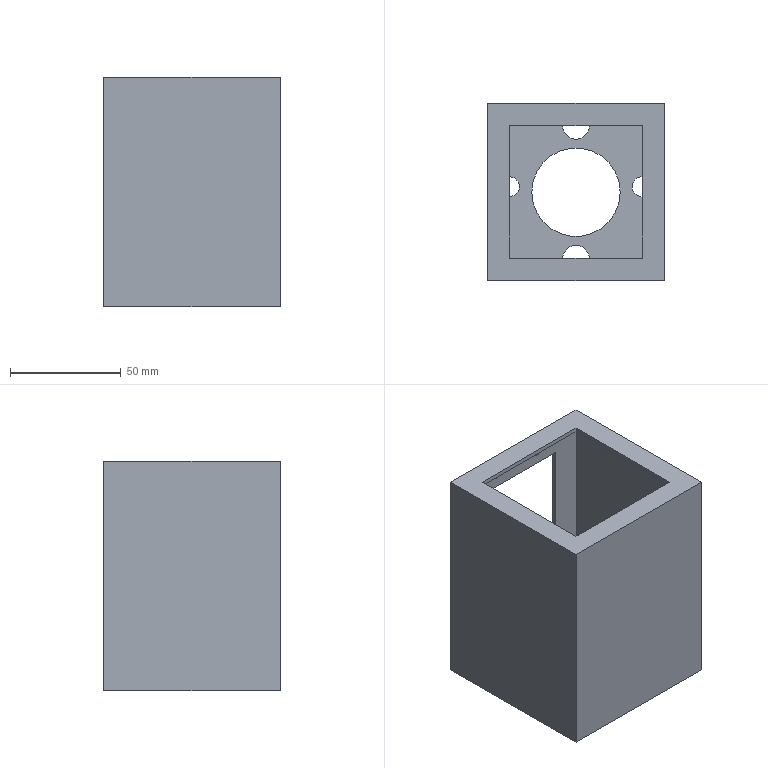Part | SolidWorks | features BaseBody 1 | 1 solid | 38 faces | box 80 x 80 x 104 mm | volume 72123 mm3 | plane 20 | cylinder 18 | commonest cylinder face diameters 3 x8 9 x4 12 x4 40 x2
STEP:
#1=CARTESIAN_POINT('',(6.,-30.,2.));
#2=VERTEX_POINT('',#1);
#3=CARTESIAN_POINT('',(-6.,-30.,2.));
#4=VERTEX_POINT('',#3);
#5=CARTESIAN_POINT('',(0.,-30.,2.));
#6=DIRECTION('',(0.,0.,-1.));
#7=DIRECTION('',(-1.,0.,0.));
#8=AXIS2_PLACEMENT_3D('',#5,#6,#7);
#9=CIRCLE('',#8,6.);
#10=EDGE_CURVE('',#2,#4,#9,.T.);
#11=ORIENTED_EDGE('',*,*,#10,.F.);
#12=CARTESIAN_POINT('',(6.,-30.,0.));
#13=VERTEX_POINT('',#12);
#14=CARTESIAN_POINT('',(6.,-30.,2.));
#15=DIRECTION('',(0.,0.,-1.));
#16=VECTOR('',#15,1000.);
#17=LINE('',#14,#16);
#18=EDGE_CURVE('',#2,#13,#17,.T.);
#19=ORIENTED_EDGE('',*,*,#18,.T.);
#20=CARTESIAN_POINT('',(-6.,-30.,0.));
#21=VERTEX_POINT('',#20);
#22=CARTESIAN_POINT('',(0.,-30.,0.));
#23=DIRECTION('',(0.,0.,1.));
#24=DIRECTION('',(-1.,0.,0.));
#25=AXIS2_PLACEMENT_3D('',#22,#23,#24);
#26=CIRCLE('',#25,6.);
#27=EDGE_CURVE('',#21,#13,#26,.T.);
#28=ORIENTED_EDGE('',*,*,#27,.F.);
#29=CARTESIAN_POINT('',(-6.,-30.,2.));
#30=DIRECTION('',(0.,0.,-1.));
#31=VECTOR('',#30,1000.);
#32=LINE('',#29,#31);
#33=EDGE_CURVE('',#4,#21,#32,.T.);
#34=ORIENTED_EDGE('',*,*,#33,.F.);
#35=EDGE_LOOP('',(#11,#19,#28,#34));
#36=FACE_OUTER_BOUND('',#35,.T.);
#37=CARTESIAN_POINT('',(0.,-30.,2.));
#38=DIRECTION('',(0.,0.,-1.));
#39=DIRECTION('',(-1.,0.,0.));
#40=AXIS2_PLACEMENT_3D('',#37,#38,#39);
#41=CYLINDRICAL_SURFACE('',#40,6.);
#42=ADVANCED_FACE('',(#36),#41,.F.);
#43=CARTESIAN_POINT('',(34.396,2.5,2.));
#44=VERTEX_POINT('',#43);
#45=CARTESIAN_POINT('',(25.396,2.5,2.));
#46=VERTEX_POINT('',#45);
#47=CARTESIAN_POINT('',(29.896,2.5,2.));
#48=DIRECTION('',(0.,0.,-1.));
#49=DIRECTION('',(-1.,0.,0.));
#50=AXIS2_PLACEMENT_3D('',#47,#48,#49);
#51=CIRCLE('',#50,4.5);
#52=EDGE_CURVE('',#44,#46,#51,.T.);
#53=ORIENTED_EDGE('',*,*,#52,.F.);
#54=CARTESIAN_POINT('',(34.396,2.5,0.));
#55=VERTEX_POINT('',#54);
#56=CARTESIAN_POINT('',(34.396,2.5,2.));
#57=DIRECTION('',(0.,0.,-1.));
#58=VECTOR('',#57,1000.);
#59=LINE('',#56,#58);
#60=EDGE_CURVE('',#44,#55,#59,.T.);
#61=ORIENTED_EDGE('',*,*,#60,.T.);
#62=CARTESIAN_POINT('',(25.396,2.5,0.));
#63=VERTEX_POINT('',#62);
#64=CARTESIAN_POINT('',(29.896,2.5,0.));
#65=DIRECTION('',(0.,0.,1.));
#66=DIRECTION('',(-1.,0.,0.));
#67=AXIS2_PLACEMENT_3D('',#64,#65,#66);
#68=CIRCLE('',#67,4.5);
#69=EDGE_CURVE('',#63,#55,#68,.T.);
#70=ORIENTED_EDGE('',*,*,#69,.F.);
#71=CARTESIAN_POINT('',(25.396,2.5,2.));
#72=DIRECTION('',(0.,0.,-1.));
#73=VECTOR('',#72,1000.);
#74=LINE('',#71,#73);
#75=EDGE_CURVE('',#46,#63,#74,.T.);
#76=ORIENTED_EDGE('',*,*,#75,.F.);
#77=EDGE_LOOP('',(#53,#61,#70,#76));
#78=FACE_OUTER_BOUND('',#77,.T.);
#79=CARTESIAN_POINT('',(29.896,2.5,2.));
#80=DIRECTION('',(0.,0.,-1.));
#81=DIRECTION('',(-1.,0.,0.));
#82=AXIS2_PLACEMENT_3D('',#79,#80,#81);
#83=CYLINDRICAL_SURFACE('',#82,4.5);
#84=ADVANCED_FACE('',(#78),#83,.F.);
#85=CARTESIAN_POINT('',(20.,0.,2.));
#86=VERTEX_POINT('',#85);
#87=CARTESIAN_POINT('',(-20.,0.,2.));
#88=VERTEX_POINT('',#87);
#89=CARTESIAN_POINT('',(0.,0.,2.));
#90=DIRECTION('',(0.,0.,-1.));
#91=DIRECTION('',(-1.,0.,0.));
#92=AXIS2_PLACEMENT_3D('',#89,#90,#91);
#93=CIRCLE('',#92,20.);
#94=EDGE_CURVE('',#86,#88,#93,.T.);
#95=ORIENTED_EDGE('',*,*,#94,.F.);
#96=CARTESIAN_POINT('',(20.,0.,0.));
#97=VERTEX_POINT('',#96);
#98=CARTESIAN_POINT('',(20.,0.,2.));
#99=DIRECTION('',(0.,0.,-1.));
#100=VECTOR('',#99,1000.);
#101=LINE('',#98,#100);
#102=EDGE_CURVE('',#86,#97,#101,.T.);
#103=ORIENTED_EDGE('',*,*,#102,.T.);
#104=CARTESIAN_POINT('',(-20.,0.,0.));
#105=VERTEX_POINT('',#104);
#106=CARTESIAN_POINT('',(0.,0.,0.));
#107=DIRECTION('',(0.,0.,1.));
#108=DIRECTION('',(-1.,0.,0.));
#109=AXIS2_PLACEMENT_3D('',#106,#107,#108);
#110=CIRCLE('',#109,20.);
#111=EDGE_CURVE('',#105,#97,#110,.T.);
#112=ORIENTED_EDGE('',*,*,#111,.F.);
#113=CARTESIAN_POINT('',(-20.,0.,2.));
#114=DIRECTION('',(0.,0.,-1.));
#115=VECTOR('',#114,1000.);
#116=LINE('',#113,#115);
#117=EDGE_CURVE('',#88,#105,#116,.T.);
#118=ORIENTED_EDGE('',*,*,#117,.F.);
#119=EDGE_LOOP('',(#95,#103,#112,#118));
#120=FACE_OUTER_BOUND('',#119,.T.);
#121=CARTESIAN_POINT('',(0.,0.,2.));
#122=DIRECTION('',(0.,0.,-1.));
#123=DIRECTION('',(-1.,0.,0.));
#124=AXIS2_PLACEMENT_3D('',#121,#122,#123);
#125=CYLINDRICAL_SURFACE('',#124,20.);
#126=ADVANCED_FACE('',(#120),#125,.F.);
#127=CARTESIAN_POINT('',(-25.604,2.5,2.));
#128=VERTEX_POINT('',#127);
#129=CARTESIAN_POINT('',(-34.604,2.5,2.));
#130=VERTEX_POINT('',#129);
#131=CARTESIAN_POINT('',(-30.104,2.5,2.));
#132=DIRECTION('',(0.,0.,-1.));
#133=DIRECTION('',(-1.,0.,0.));
#134=AXIS2_PLACEMENT_3D('',#131,#132,#133);
#135=CIRCLE('',#134,4.5);
#136=EDGE_CURVE('',#128,#130,#135,.T.);
#137=ORIENTED_EDGE('',*,*,#136,.F.);
#138=CARTESIAN_POINT('',(-25.604,2.5,0.));
#139=VERTEX_POINT('',#138);
#140=CARTESIAN_POINT('',(-25.604,2.5,2.));
#141=DIRECTION('',(0.,0.,-1.));
#142=VECTOR('',#141,1000.);
#143=LINE('',#140,#142);
#144=EDGE_CURVE('',#128,#139,#143,.T.);
#145=ORIENTED_EDGE('',*,*,#144,.T.);
#146=CARTESIAN_POINT('',(-34.604,2.5,0.));
#147=VERTEX_POINT('',#146);
#148=CARTESIAN_POINT('',(-30.104,2.5,0.));
#149=DIRECTION('',(0.,0.,1.));
#150=DIRECTION('',(-1.,0.,0.));
#151=AXIS2_PLACEMENT_3D('',#148,#149,#150);
#152=CIRCLE('',#151,4.5);
#153=EDGE_CURVE('',#147,#139,#152,.T.);
#154=ORIENTED_EDGE('',*,*,#153,.F.);
#155=CARTESIAN_POINT('',(-34.604,2.5,2.));
#156=DIRECTION('',(0.,0.,-1.));
#157=VECTOR('',#156,1000.);
#158=LINE('',#155,#157);
#159=EDGE_CURVE('',#130,#147,#158,.T.);
#160=ORIENTED_EDGE('',*,*,#159,.F.);
#161=EDGE_LOOP('',(#137,#145,#154,#160));
#162=FACE_OUTER_BOUND('',#161,.T.);
#163=CARTESIAN_POINT('',(-30.104,2.5,2.));
#164=DIRECTION('',(0.,0.,-1.));
#165=DIRECTION('',(-1.,0.,0.));
#166=AXIS2_PLACEMENT_3D('',#163,#164,#165);
#167=CYLINDRICAL_SURFACE('',#166,4.5);
#168=ADVANCED_FACE('',(#162),#167,.F.);
#169=CARTESIAN_POINT('',(6.,30.,2.));
#170=VERTEX_POINT('',#169);
#171=CARTESIAN_POINT('',(-6.,30.,2.));
#172=VERTEX_POINT('',#171);
#173=CARTESIAN_POINT('',(0.,30.,2.));
#174=DIRECTION('',(0.,0.,-1.));
#175=DIRECTION('',(-1.,0.,0.));
#176=AXIS2_PLACEMENT_3D('',#173,#174,#175);
#177=CIRCLE('',#176,6.);
#178=EDGE_CURVE('',#170,#172,#177,.T.);
#179=ORIENTED_EDGE('',*,*,#178,.F.);
#180=CARTESIAN_POINT('',(6.,30.,0.));
#181=VERTEX_POINT('',#180);
#182=CARTESIAN_POINT('',(6.,30.,2.));
#183=DIRECTION('',(0.,0.,-1.));
#184=VECTOR('',#183,1000.);
#185=LINE('',#182,#184);
#186=EDGE_CURVE('',#170,#181,#185,.T.);
#187=ORIENTED_EDGE('',*,*,#186,.T.);
#188=CARTESIAN_POINT('',(-6.,30.,0.));
#189=VERTEX_POINT('',#188);
#190=CARTESIAN_POINT('',(0.,30.,0.));
#191=DIRECTION('',(0.,0.,1.));
#192=DIRECTION('',(-1.,0.,0.));
#193=AXIS2_PLACEMENT_3D('',#190,#191,#192);
#194=CIRCLE('',#193,6.);
#195=EDGE_CURVE('',#189,#181,#194,.T.);
#196=ORIENTED_EDGE('',*,*,#195,.F.);
#197=CARTESIAN_POINT('',(-6.,30.,2.));
#198=DIRECTION('',(0.,0.,-1.));
#199=VECTOR('',#198,1000.);
#200=LINE('',#197,#199);
#201=EDGE_CURVE('',#172,#189,#200,.T.);
#202=ORIENTED_EDGE('',*,*,#201,.F.);
#203=EDGE_LOOP('',(#179,#187,#196,#202));
#204=FACE_OUTER_BOUND('',#203,.T.);
#205=CARTESIAN_POINT('',(0.,30.,2.));
#206=DIRECTION('',(0.,0.,-1.));
#207=DIRECTION('',(-1.,0.,0.));
#208=AXIS2_PLACEMENT_3D('',#205,#206,#207);
#209=CYLINDRICAL_SURFACE('',#208,6.);
#210=ADVANCED_FACE('',(#204),#209,.F.);
#211=CARTESIAN_POINT('',(-13.,38.,93.5));
#212=VERTEX_POINT('',#211);
#213=CARTESIAN_POINT('',(-13.,38.,96.5));
#214=VERTEX_POINT('',#213);
#215=CARTESIAN_POINT('',(-13.,38.,95.));
#216=DIRECTION('',(0.,1.,0.));
#217=DIRECTION('',(0.,0.,1.));
#218=AXIS2_PLACEMENT_3D('',#215,#216,#217);
#219=CIRCLE('',#218,1.5);
#220=EDGE_CURVE('',#212,#214,#219,.T.);
#221=ORIENTED_EDGE('',*,*,#220,.F.);
#222=CARTESIAN_POINT('',(-13.,40.,93.5));
#223=VERTEX_POINT('',#222);
#224=CARTESIAN_POINT('',(-13.,35.,93.5));
#225=DIRECTION('',(0.,1.,0.));
#226=VECTOR('',#225,1000.);
#227=LINE('',#224,#226);
#228=EDGE_CURVE('',#212,#223,#227,.T.);
#229=ORIENTED_EDGE('',*,*,#228,.T.);
#230=CARTESIAN_POINT('',(-13.,40.,96.5));
#231=VERTEX_POINT('',#230);
#232=CARTESIAN_POINT('',(-13.,40.,95.));
#233=DIRECTION('',(0.,1.,0.));
#234=DIRECTION('',(0.,0.,1.));
#235=AXIS2_PLACEMENT_3D('',#232,#233,#234);
#236=CIRCLE('',#235,1.5);
#237=EDGE_CURVE('',#223,#231,#236,.T.);
#238=ORIENTED_EDGE('',*,*,#237,.T.);
#239=CARTESIAN_POINT('',(-13.,35.,96.5));
#240=DIRECTION('',(0.,1.,0.));
#241=VECTOR('',#240,1000.);
#242=LINE('',#239,#241);
#243=EDGE_CURVE('',#214,#231,#242,.T.);
#244=ORIENTED_EDGE('',*,*,#243,.F.);
#245=EDGE_LOOP('',(#221,#229,#238,#244));
#246=FACE_OUTER_BOUND('',#245,.T.);
#247=CARTESIAN_POINT('',(-13.,35.,95.));
#248=DIRECTION('',(0.,1.,0.));
#249=DIRECTION('',(0.,0.,1.));
#250=AXIS2_PLACEMENT_3D('',#247,#248,#249);
#251=CYLINDRICAL_SURFACE('',#250,1.5);
#252=ADVANCED_FACE('',(#246),#251,.F.);
#253=CARTESIAN_POINT('',(13.,38.,93.5));
#254=VERTEX_POINT('',#253);
#255=CARTESIAN_POINT('',(13.,38.,96.5));
#256=VERTEX_POINT('',#255);
#257=CARTESIAN_POINT('',(13.,38.,95.));
#258=DIRECTION('',(0.,1.,0.));
#259=DIRECTION('',(0.,0.,1.));
#260=AXIS2_PLACEMENT_3D('',#257,#258,#259);
#261=CIRCLE('',#260,1.5);
#262=EDGE_CURVE('',#254,#256,#261,.T.);
#263=ORIENTED_EDGE('',*,*,#262,.F.);
#264=CARTESIAN_POINT('',(13.,40.,93.5));
#265=VERTEX_POINT('',#264);
#266=CARTESIAN_POINT('',(13.,35.,93.5));
#267=DIRECTION('',(0.,1.,0.));
#268=VECTOR('',#267,1000.);
#269=LINE('',#266,#268);
#270=EDGE_CURVE('',#254,#265,#269,.T.);
#271=ORIENTED_EDGE('',*,*,#270,.T.);
#272=CARTESIAN_POINT('',(13.,40.,96.5));
#273=VERTEX_POINT('',#272);
#274=CARTESIAN_POINT('',(13.,40.,95.));
#275=DIRECTION('',(0.,1.,0.));
#276=DIRECTION('',(0.,0.,1.));
#277=AXIS2_PLACEMENT_3D('',#274,#275,#276);
#278=CIRCLE('',#277,1.5);
#279=EDGE_CURVE('',#265,#273,#278,.T.);
#280=ORIENTED_EDGE('',*,*,#279,.T.);
#281=CARTESIAN_POINT('',(13.,35.,96.5));
#282=DIRECTION('',(0.,1.,0.));
#283=VECTOR('',#282,1000.);
#284=LINE('',#281,#283);
#285=EDGE_CURVE('',#256,#273,#284,.T.);
#286=ORIENTED_EDGE('',*,*,#285,.F.);
#287=EDGE_LOOP('',(#263,#271,#280,#286));
#288=FACE_OUTER_BOUND('',#287,.T.);
#289=CARTESIAN_POINT('',(13.,35.,95.));
#290=DIRECTION('',(0.,1.,0.));
#291=DIRECTION('',(0.,0.,1.));
#292=AXIS2_PLACEMENT_3D('',#289,#290,#291);
#293=CYLINDRICAL_SURFACE('',#292,1.5);
#294=ADVANCED_FACE('',(#288),#293,.F.);
#295=CARTESIAN_POINT('',(13.,38.,27.5));
#296=VERTEX_POINT('',#295);
#297=CARTESIAN_POINT('',(13.,38.,30.5));
#298=VERTEX_POINT('',#297);
#299=CARTESIAN_POINT('',(13.,38.,29.));
#300=DIRECTION('',(0.,1.,0.));
#301=DIRECTION('',(0.,0.,1.));
#302=AXIS2_PLACEMENT_3D('',#299,#300,#301);
#303=CIRCLE('',#302,1.5);
#304=EDGE_CURVE('',#296,#298,#303,.T.);
#305=ORIENTED_EDGE('',*,*,#304,.F.);
#306=CARTESIAN_POINT('',(13.,40.,27.5));
#307=VERTEX_POINT('',#306);
#308=CARTESIAN_POINT('',(13.,35.,27.5));
#309=DIRECTION('',(0.,1.,0.));
#310=VECTOR('',#309,1000.);
#311=LINE('',#308,#310);
#312=EDGE_CURVE('',#296,#307,#311,.T.);
#313=ORIENTED_EDGE('',*,*,#312,.T.);
#314=CARTESIAN_POINT('',(13.,40.,30.5));
#315=VERTEX_POINT('',#314);
#316=CARTESIAN_POINT('',(13.,40.,29.));
#317=DIRECTION('',(0.,1.,0.));
#318=DIRECTION('',(0.,0.,1.));
#319=AXIS2_PLACEMENT_3D('',#316,#317,#318);
#320=CIRCLE('',#319,1.5);
#321=EDGE_CURVE('',#307,#315,#320,.T.);
#322=ORIENTED_EDGE('',*,*,#321,.T.);
#323=CARTESIAN_POINT('',(13.,35.,30.5));
#324=DIRECTION('',(0.,1.,0.));
#325=VECTOR('',#324,1000.);
#326=LINE('',#323,#325);
#327=EDGE_CURVE('',#298,#315,#326,.T.);
#328=ORIENTED_EDGE('',*,*,#327,.F.);
#329=EDGE_LOOP('',(#305,#313,#322,#328));
#330=FACE_OUTER_BOUND('',#329,.T.);
#331=CARTESIAN_POINT('',(13.,35.,29.));
#332=DIRECTION('',(0.,1.,0.));
#333=DIRECTION('',(0.,0.,1.));
#334=AXIS2_PLACEMENT_3D('',#331,#332,#333);
#335=CYLINDRICAL_SURFACE('',#334,1.5);
#336=ADVANCED_FACE('',(#330),#335,.F.);
#337=CARTESIAN_POINT('',(-13.,38.,27.5));
#338=VERTEX_POINT('',#337);
#339=CARTESIAN_POINT('',(-13.,38.,30.5));
#340=VERTEX_POINT('',#339);
#341=CARTESIAN_POINT('',(-13.,38.,29.));
#342=DIRECTION('',(0.,1.,0.));
#343=DIRECTION('',(0.,0.,1.));
#344=AXIS2_PLACEMENT_3D('',#341,#342,#343);
#345=CIRCLE('',#344,1.5);
#346=EDGE_CURVE('',#338,#340,#345,.T.);
#347=ORIENTED_EDGE('',*,*,#346,.F.);
#348=CARTESIAN_POINT('',(-13.,40.,27.5));
#349=VERTEX_POINT('',#348);
#350=CARTESIAN_POINT('',(-13.,35.,27.5));
#351=DIRECTION('',(0.,1.,0.));
#352=VECTOR('',#351,1000.);
#353=LINE('',#350,#352);
#354=EDGE_CURVE('',#338,#349,#353,.T.);
#355=ORIENTED_EDGE('',*,*,#354,.T.);
#356=CARTESIAN_POINT('',(-13.,40.,30.5));
#357=VERTEX_POINT('',#356);
#358=CARTESIAN_POINT('',(-13.,40.,29.));
#359=DIRECTION('',(0.,1.,0.));
#360=DIRECTION('',(0.,0.,1.));
#361=AXIS2_PLACEMENT_3D('',#358,#359,#360);
#362=CIRCLE('',#361,1.5);
#363=EDGE_CURVE('',#349,#357,#362,.T.);
#364=ORIENTED_EDGE('',*,*,#363,.T.);
#365=CARTESIAN_POINT('',(-13.,35.,30.5));
#366=DIRECTION('',(0.,1.,0.));
#367=VECTOR('',#366,1000.);
#368=LINE('',#365,#367);
#369=EDGE_CURVE('',#340,#357,#368,.T.);
#370=ORIENTED_EDGE('',*,*,#369,.F.);
#371=EDGE_LOOP('',(#347,#355,#364,#370));
#372=FACE_OUTER_BOUND('',#371,.T.);
#373=CARTESIAN_POINT('',(-13.,35.,29.));
#374=DIRECTION('',(0.,1.,0.));
#375=DIRECTION('',(0.,0.,1.));
#376=AXIS2_PLACEMENT_3D('',#373,#374,#375);
#377=CYLINDRICAL_SURFACE('',#376,1.5);
#378=ADVANCED_FACE('',(#372),#377,.F.);
#379=CARTESIAN_POINT('',(-40.,-40.,104.));
#380=VERTEX_POINT('',#379);
#381=CARTESIAN_POINT('',(-40.,-40.,0.));
#382=VERTEX_POINT('',#381);
#383=CARTESIAN_POINT('',(-40.,-40.,2.));
#384=DIRECTION('',(0.,0.,-1.));
#385=VECTOR('',#384,1000.);
#386=LINE('',#383,#385);
#387=EDGE_CURVE('',#380,#382,#386,.T.);
#388=ORIENTED_EDGE('',*,*,#387,.F.);
#389=CARTESIAN_POINT('',(-40.,40.,104.));
#390=VERTEX_POINT('',#389);
#391=CARTESIAN_POINT('',(-40.,40.,104.));
#392=DIRECTION('',(0.,-1.,0.));
#393=VECTOR('',#392,1000.);
#394=LINE('',#391,#393);
#395=EDGE_CURVE('',#390,#380,#394,.T.);
#396=ORIENTED_EDGE('',*,*,#395,.F.);
#397=CARTESIAN_POINT('',(-40.,40.,0.));
#398=VERTEX_POINT('',#397);
#399=CARTESIAN_POINT('',(-40.,40.,2.));
#400=DIRECTION('',(0.,0.,1.));
#401=VECTOR('',#400,1000.);
#402=LINE('',#399,#401);
#403=EDGE_CURVE('',#398,#390,#402,.T.);
#404=ORIENTED_EDGE('',*,*,#403,.F.);
#405=CARTESIAN_POINT('',(-40.,40.,0.));
#406=DIRECTION('',(0.,1.,0.));
#407=VECTOR('',#406,1000.);
#408=LINE('',#405,#407);
#409=EDGE_CURVE('',#382,#398,#408,.T.);
#410=ORIENTED_EDGE('',*,*,#409,.F.);
#411=EDGE_LOOP('',(#388,#396,#404,#410));
#412=FACE_OUTER_BOUND('',#411,.T.);
#413=CARTESIAN_POINT('',(-40.,40.,2.));
#414=DIRECTION('',(1.,0.,0.));
#415=DIRECTION('',(0.,1.,0.));
#416=AXIS2_PLACEMENT_3D('',#413,#414,#415);
#417=PLANE('',#416);
#418=ADVANCED_FACE('',(#412),#417,.F.);
#419=ORIENTED_EDGE('',*,*,#27,.T.);
#420=CARTESIAN_POINT('',(0.,-30.,0.));
#421=DIRECTION('',(0.,0.,1.));
#422=DIRECTION('',(-1.,0.,0.));
#423=AXIS2_PLACEMENT_3D('',#420,#421,#422);
#424=CIRCLE('',#423,6.);
#425=EDGE_CURVE('',#13,#21,#424,.T.);
#426=ORIENTED_EDGE('',*,*,#425,.T.);
#427=EDGE_LOOP('',(#419,#426));
#428=FACE_BOUND('',#427,.T.);
#429=ORIENTED_EDGE('',*,*,#69,.T.);
#430=CARTESIAN_POINT('',(29.896,2.5,0.));
#431=DIRECTION('',(0.,0.,1.));
#432=DIRECTION('',(-1.,0.,0.));
#433=AXIS2_PLACEMENT_3D('',#430,#431,#432);
#434=CIRCLE('',#433,4.5);
#435=EDGE_CURVE('',#55,#63,#434,.T.);
#436=ORIENTED_EDGE('',*,*,#435,.T.);
#437=EDGE_LOOP('',(#429,#436));
#438=FACE_BOUND('',#437,.T.);
#439=ORIENTED_EDGE('',*,*,#111,.T.);
#440=CARTESIAN_POINT('',(0.,0.,0.));
#441=DIRECTION('',(0.,0.,1.));
#442=DIRECTION('',(-1.,0.,0.));
#443=AXIS2_PLACEMENT_3D('',#440,#441,#442);
#444=CIRCLE('',#443,20.);
#445=EDGE_CURVE('',#97,#105,#444,.T.);
#446=ORIENTED_EDGE('',*,*,#445,.T.);
#447=EDGE_LOOP('',(#439,#446));
#448=FACE_BOUND('',#447,.T.);
#449=ORIENTED_EDGE('',*,*,#153,.T.);
#450=CARTESIAN_POINT('',(-30.104,2.5,0.));
#451=DIRECTION('',(0.,0.,1.));
#452=DIRECTION('',(-1.,0.,0.));
#453=AXIS2_PLACEMENT_3D('',#450,#451,#452);
#454=CIRCLE('',#453,4.5);
#455=EDGE_CURVE('',#139,#147,#454,.T.);
#456=ORIENTED_EDGE('',*,*,#455,.T.);
#457=EDGE_LOOP('',(#449,#456));
#458=FACE_BOUND('',#457,.T.);
#459=ORIENTED_EDGE('',*,*,#195,.T.);
#460=CARTESIAN_POINT('',(0.,30.,0.));
#461=DIRECTION('',(0.,0.,1.));
#462=DIRECTION('',(-1.,0.,0.));
#463=AXIS2_PLACEMENT_3D('',#460,#461,#462);
#464=CIRCLE('',#463,6.);
#465=EDGE_CURVE('',#181,#189,#464,.T.);
#466=ORIENTED_EDGE('',*,*,#465,.T.);
#467=EDGE_LOOP('',(#459,#466));
#468=FACE_BOUND('',#467,.T.);
#469=CARTESIAN_POINT('',(40.,40.,0.));
#470=VERTEX_POINT('',#469);
#471=CARTESIAN_POINT('',(40.,-40.,0.));
#472=VERTEX_POINT('',#471);
#473=CARTESIAN_POINT('',(40.,0.,0.));
#474=DIRECTION('',(0.,-1.,0.));
#475=VECTOR('',#474,1000.);
#476=LINE('',#473,#475);
#477=EDGE_CURVE('',#470,#472,#476,.T.);
#478=ORIENTED_EDGE('',*,*,#477,.T.);
#479=CARTESIAN_POINT('',(0.,-40.,0.));
#480=DIRECTION('',(-1.,0.,0.));
#481=VECTOR('',#480,1000.);
#482=LINE('',#479,#481);
#483=EDGE_CURVE('',#472,#382,#482,.T.);
#484=ORIENTED_EDGE('',*,*,#483,.T.);
#485=ORIENTED_EDGE('',*,*,#409,.T.);
#486=CARTESIAN_POINT('',(0.,40.,0.));
#487=DIRECTION('',(1.,0.,0.));
#488=VECTOR('',#487,1000.);
#489=LINE('',#486,#488);
#490=EDGE_CURVE('',#398,#470,#489,.T.);
#491=ORIENTED_EDGE('',*,*,#490,.T.);
#492=EDGE_LOOP('',(#478,#484,#485,#491));
#493=FACE_OUTER_BOUND('',#492,.T.);
#494=CARTESIAN_POINT('',(0.,0.,0.));
#495=DIRECTION('',(0.,0.,-1.));
#496=DIRECTION('',(-1.,0.,0.));
#497=AXIS2_PLACEMENT_3D('',#494,#495,#496);
#498=PLANE('',#497);
#499=ADVANCED_FACE('',(#428,#438,#448,#458,#468,#493),#498,.T.);
#500=CARTESIAN_POINT('',(40.,-40.,104.));
#501=VERTEX_POINT('',#500);
#502=CARTESIAN_POINT('',(40.,-40.,2.));
#503=DIRECTION('',(0.,0.,-1.));
#504=VECTOR('',#503,1000.);
#505=LINE('',#502,#504);
#506=EDGE_CURVE('',#501,#472,#505,.T.);
#507=ORIENTED_EDGE('',*,*,#506,.F.);
#508=CARTESIAN_POINT('',(40.,-40.,104.));
#509=DIRECTION('',(1.,0.,0.));
#510=VECTOR('',#509,1000.);
#511=LINE('',#508,#510);
#512=EDGE_CURVE('',#380,#501,#511,.T.);
#513=ORIENTED_EDGE('',*,*,#512,.F.);
#514=ORIENTED_EDGE('',*,*,#387,.T.);
#515=ORIENTED_EDGE('',*,*,#483,.F.);
#516=EDGE_LOOP('',(#507,#513,#514,#515));
#517=FACE_OUTER_BOUND('',#516,.T.);
#518=CARTESIAN_POINT('',(40.,-40.,2.));
#519=DIRECTION('',(0.,1.,0.));
#520=DIRECTION('',(-1.,0.,0.));
#521=AXIS2_PLACEMENT_3D('',#518,#519,#520);
#522=PLANE('',#521);
#523=ADVANCED_FACE('',(#517),#522,.F.);
#524=CARTESIAN_POINT('',(-30.,30.,104.));
#525=VERTEX_POINT('',#524);
#526=CARTESIAN_POINT('',(30.,30.,104.));
#527=VERTEX_POINT('',#526);
#528=CARTESIAN_POINT('',(0.,30.,104.));
#529=DIRECTION('',(1.,0.,0.));
#530=VECTOR('',#529,1000.);
#531=LINE('',#528,#530);
#532=EDGE_CURVE('',#525,#527,#531,.T.);
#533=ORIENTED_EDGE('',*,*,#532,.T.);
#534=CARTESIAN_POINT('',(30.,-30.,104.));
#535=VERTEX_POINT('',#534);
#536=CARTESIAN_POINT('',(30.,0.,104.));
#537=DIRECTION('',(0.,-1.,0.));
#538=VECTOR('',#537,1000.);
#539=LINE('',#536,#538);
#540=EDGE_CURVE('',#527,#535,#539,.T.);
#541=ORIENTED_EDGE('',*,*,#540,.T.);
#542=CARTESIAN_POINT('',(-30.,-30.,104.));
#543=VERTEX_POINT('',#542);
#544=CARTESIAN_POINT('',(0.,-30.,104.));
#545=DIRECTION('',(-1.,0.,0.));
#546=VECTOR('',#545,1000.);
#547=LINE('',#544,#546);
#548=EDGE_CURVE('',#535,#543,#547,.T.);
#549=ORIENTED_EDGE('',*,*,#548,.T.);
#550=CARTESIAN_POINT('',(-30.,0.,104.));
#551=DIRECTION('',(0.,1.,0.));
#552=VECTOR('',#551,1000.);
#553=LINE('',#550,#552);
#554=EDGE_CURVE('',#543,#525,#553,.T.);
#555=ORIENTED_EDGE('',*,*,#554,.T.);
#556=EDGE_LOOP('',(#533,#541,#549,#555));
#557=FACE_BOUND('',#556,.T.);
#558=CARTESIAN_POINT('',(40.,40.,104.));
#559=VERTEX_POINT('',#558);
#560=CARTESIAN_POINT('',(40.,0.,104.));
#561=DIRECTION('',(0.,1.,0.));
#562=VECTOR('',#561,1000.);
#563=LINE('',#560,#562);
#564=EDGE_CURVE('',#501,#559,#563,.T.);
#565=ORIENTED_EDGE('',*,*,#564,.T.);
#566=CARTESIAN_POINT('',(0.,40.,104.));
#567=DIRECTION('',(-1.,0.,0.));
#568=VECTOR('',#567,1000.);
#569=LINE('',#566,#568);
#570=EDGE_CURVE('',#559,#390,#569,.T.);
#571=ORIENTED_EDGE('',*,*,#570,.T.);
#572=ORIENTED_EDGE('',*,*,#395,.T.);
#573=ORIENTED_EDGE('',*,*,#512,.T.);
#574=EDGE_LOOP('',(#565,#571,#572,#573));
#575=FACE_OUTER_BOUND('',#574,.T.);
#576=CARTESIAN_POINT('',(0.,0.,104.));
#577=DIRECTION('',(0.,0.,1.));
#578=DIRECTION('',(1.,0.,0.));
#579=AXIS2_PLACEMENT_3D('',#576,#577,#578);
#580=PLANE('',#579);
#581=ADVANCED_FACE('',(#557,#575),#580,.T.);
#582=CARTESIAN_POINT('',(-25.,40.,35.));
#583=VERTEX_POINT('',#582);
#584=CARTESIAN_POINT('',(-25.,40.,89.));
#585=VERTEX_POINT('',#584);
#586=CARTESIAN_POINT('',(-25.,40.,2.));
#587=DIRECTION('',(0.,0.,1.));
#588=VECTOR('',#587,1000.);
#589=LINE('',#586,#588);
#590=EDGE_CURVE('',#583,#585,#589,.T.);
#591=ORIENTED_EDGE('',*,*,#590,.F.);
#592=CARTESIAN_POINT('',(25.,40.,35.));
#593=VERTEX_POINT('',#592);
#594=CARTESIAN_POINT('',(40.,40.,35.));
#595=DIRECTION('',(-1.,0.,0.));
#596=VECTOR('',#595,1000.);
#597=LINE('',#594,#596);
#598=EDGE_CURVE('',#593,#583,#597,.T.);
#599=ORIENTED_EDGE('',*,*,#598,.F.);
#600=CARTESIAN_POINT('',(25.,40.,89.));
#601=VERTEX_POINT('',#600);
#602=CARTESIAN_POINT('',(25.,40.,2.));
#603=DIRECTION('',(0.,0.,-1.));
#604=VECTOR('',#603,1000.);
#605=LINE('',#602,#604);
#606=EDGE_CURVE('',#601,#593,#605,.T.);
#607=ORIENTED_EDGE('',*,*,#606,.F.);
#608=CARTESIAN_POINT('',(40.,40.,89.));
#609=DIRECTION('',(1.,0.,0.));
#610=VECTOR('',#609,1000.);
#611=LINE('',#608,#610);
#612=EDGE_CURVE('',#585,#601,#611,.T.);
#613=ORIENTED_EDGE('',*,*,#612,.F.);
#614=EDGE_LOOP('',(#591,#599,#607,#613));
#615=FACE_BOUND('',#614,.T.);
#616=CARTESIAN_POINT('',(-13.,40.,95.));
#617=DIRECTION('',(0.,1.,0.));
#618=DIRECTION('',(0.,0.,1.));
#619=AXIS2_PLACEMENT_3D('',#616,#617,#618);
#620=CIRCLE('',#619,1.5);
#621=EDGE_CURVE('',#231,#223,#620,.T.);
#622=ORIENTED_EDGE('',*,*,#621,.F.);
#623=ORIENTED_EDGE('',*,*,#237,.F.);
#624=EDGE_LOOP('',(#622,#623));
#625=FACE_BOUND('',#624,.T.);
#626=CARTESIAN_POINT('',(13.,40.,95.));
#627=DIRECTION('',(0.,1.,0.));
#628=DIRECTION('',(0.,0.,1.));
#629=AXIS2_PLACEMENT_3D('',#626,#627,#628);
#630=CIRCLE('',#629,1.5);
#631=EDGE_CURVE('',#273,#265,#630,.T.);
#632=ORIENTED_EDGE('',*,*,#631,.F.);
#633=ORIENTED_EDGE('',*,*,#279,.F.);
#634=EDGE_LOOP('',(#632,#633));
#635=FACE_BOUND('',#634,.T.);
#636=CARTESIAN_POINT('',(13.,40.,29.));
#637=DIRECTION('',(0.,1.,0.));
#638=DIRECTION('',(0.,0.,1.));
#639=AXIS2_PLACEMENT_3D('',#636,#637,#638);
#640=CIRCLE('',#639,1.5);
#641=EDGE_CURVE('',#315,#307,#640,.T.);
#642=ORIENTED_EDGE('',*,*,#641,.F.);
#643=ORIENTED_EDGE('',*,*,#321,.F.);
#644=EDGE_LOOP('',(#642,#643));
#645=FACE_BOUND('',#644,.T.);
#646=CARTESIAN_POINT('',(-13.,40.,29.));
#647=DIRECTION('',(0.,1.,0.));
#648=DIRECTION('',(0.,0.,1.));
#649=AXIS2_PLACEMENT_3D('',#646,#647,#648);
#650=CIRCLE('',#649,1.5);
#651=EDGE_CURVE('',#357,#349,#650,.T.);
#652=ORIENTED_EDGE('',*,*,#651,.F.);
#653=ORIENTED_EDGE('',*,*,#363,.F.);
#654=EDGE_LOOP('',(#652,#653));
#655=FACE_BOUND('',#654,.T.);
#656=ORIENTED_EDGE('',*,*,#403,.T.);
#657=ORIENTED_EDGE('',*,*,#570,.F.);
#658=CARTESIAN_POINT('',(40.,40.,2.));
#659=DIRECTION('',(0.,0.,1.));
#660=VECTOR('',#659,1000.);
#661=LINE('',#658,#660);
#662=EDGE_CURVE('',#470,#559,#661,.T.);
#663=ORIENTED_EDGE('',*,*,#662,.F.);
#664=ORIENTED_EDGE('',*,*,#490,.F.);
#665=EDGE_LOOP('',(#656,#657,#663,#664));
#666=FACE_OUTER_BOUND('',#665,.T.);
#667=CARTESIAN_POINT('',(40.,40.,2.));
#668=DIRECTION('',(0.,-1.,0.));
#669=DIRECTION('',(1.,0.,0.));
#670=AXIS2_PLACEMENT_3D('',#667,#668,#669);
#671=PLANE('',#670);
#672=ADVANCED_FACE('',(#615,#625,#635,#645,#655,#666),#671,.F.);
#673=ORIENTED_EDGE('',*,*,#18,.F.);
#674=CARTESIAN_POINT('',(0.,-30.,2.));
#675=DIRECTION('',(0.,0.,-1.));
#676=DIRECTION('',(-1.,0.,0.));
#677=AXIS2_PLACEMENT_3D('',#674,#675,#676);
#678=CIRCLE('',#677,6.);
#679=EDGE_CURVE('',#4,#2,#678,.T.);
#680=ORIENTED_EDGE('',*,*,#679,.F.);
#681=ORIENTED_EDGE('',*,*,#33,.T.);
#682=ORIENTED_EDGE('',*,*,#425,.F.);
#683=EDGE_LOOP('',(#673,#680,#681,#682));
#684=FACE_OUTER_BOUND('',#683,.T.);
#685=CARTESIAN_POINT('',(0.,-30.,2.));
#686=DIRECTION('',(0.,0.,-1.));
#687=DIRECTION('',(-1.,0.,0.));
#688=AXIS2_PLACEMENT_3D('',#685,#686,#687);
#689=CYLINDRICAL_SURFACE('',#688,6.);
#690=ADVANCED_FACE('',(#684),#689,.F.);
#691=ORIENTED_EDGE('',*,*,#60,.F.);
#692=CARTESIAN_POINT('',(29.896,2.5,2.));
#693=DIRECTION('',(0.,0.,-1.));
#694=DIRECTION('',(-1.,0.,0.));
#695=AXIS2_PLACEMENT_3D('',#692,#693,#694);
#696=CIRCLE('',#695,4.5);
#697=EDGE_CURVE('',#46,#44,#696,.T.);
#698=ORIENTED_EDGE('',*,*,#697,.F.);
#699=ORIENTED_EDGE('',*,*,#75,.T.);
#700=ORIENTED_EDGE('',*,*,#435,.F.);
#701=EDGE_LOOP('',(#691,#698,#699,#700));
#702=FACE_OUTER_BOUND('',#701,.T.);
#703=CARTESIAN_POINT('',(29.896,2.5,2.));
#704=DIRECTION('',(0.,0.,-1.));
#705=DIRECTION('',(-1.,0.,0.));
#706=AXIS2_PLACEMENT_3D('',#703,#704,#705);
#707=CYLINDRICAL_SURFACE('',#706,4.5);
#708=ADVANCED_FACE('',(#702),#707,.F.);
#709=ORIENTED_EDGE('',*,*,#102,.F.);
#710=CARTESIAN_POINT('',(0.,0.,2.));
#711=DIRECTION('',(0.,0.,-1.));
#712=DIRECTION('',(-1.,0.,0.));
#713=AXIS2_PLACEMENT_3D('',#710,#711,#712);
#714=CIRCLE('',#713,20.);
#715=EDGE_CURVE('',#88,#86,#714,.T.);
#716=ORIENTED_EDGE('',*,*,#715,.F.);
#717=ORIENTED_EDGE('',*,*,#117,.T.);
#718=ORIENTED_EDGE('',*,*,#445,.F.);
#719=EDGE_LOOP('',(#709,#716,#717,#718));
#720=FACE_OUTER_BOUND('',#719,.T.);
#721=CARTESIAN_POINT('',(0.,0.,2.));
#722=DIRECTION('',(0.,0.,-1.));
#723=DIRECTION('',(-1.,0.,0.));
#724=AXIS2_PLACEMENT_3D('',#721,#722,#723);
#725=CYLINDRICAL_SURFACE('',#724,20.);
#726=ADVANCED_FACE('',(#720),#725,.F.);
#727=ORIENTED_EDGE('',*,*,#144,.F.);
#728=CARTESIAN_POINT('',(-30.104,2.5,2.));
#729=DIRECTION('',(0.,0.,-1.));
#730=DIRECTION('',(-1.,0.,0.));
#731=AXIS2_PLACEMENT_3D('',#728,#729,#730);
#732=CIRCLE('',#731,4.5);
#733=EDGE_CURVE('',#130,#128,#732,.T.);
#734=ORIENTED_EDGE('',*,*,#733,.F.);
#735=ORIENTED_EDGE('',*,*,#159,.T.);
#736=ORIENTED_EDGE('',*,*,#455,.F.);
#737=EDGE_LOOP('',(#727,#734,#735,#736));
#738=FACE_OUTER_BOUND('',#737,.T.);
#739=CARTESIAN_POINT('',(-30.104,2.5,2.));
#740=DIRECTION('',(0.,0.,-1.));
#741=DIRECTION('',(-1.,0.,0.));
#742=AXIS2_PLACEMENT_3D('',#739,#740,#741);
#743=CYLINDRICAL_SURFACE('',#742,4.5);
#744=ADVANCED_FACE('',(#738),#743,.F.);
#745=ORIENTED_EDGE('',*,*,#186,.F.);
#746=CARTESIAN_POINT('',(0.,30.,2.));
#747=DIRECTION('',(0.,0.,-1.));
#748=DIRECTION('',(-1.,0.,0.));
#749=AXIS2_PLACEMENT_3D('',#746,#747,#748);
#750=CIRCLE('',#749,6.);
#751=EDGE_CURVE('',#172,#170,#750,.T.);
#752=ORIENTED_EDGE('',*,*,#751,.F.);
#753=ORIENTED_EDGE('',*,*,#201,.T.);
#754=ORIENTED_EDGE('',*,*,#465,.F.);
#755=EDGE_LOOP('',(#745,#752,#753,#754));
#756=FACE_OUTER_BOUND('',#755,.T.);
#757=CARTESIAN_POINT('',(0.,30.,2.));
#758=DIRECTION('',(0.,0.,-1.));
#759=DIRECTION('',(-1.,0.,0.));
#760=AXIS2_PLACEMENT_3D('',#757,#758,#759);
#761=CYLINDRICAL_SURFACE('',#760,6.);
#762=ADVANCED_FACE('',(#756),#761,.F.);
#763=ORIENTED_EDGE('',*,*,#662,.T.);
#764=ORIENTED_EDGE('',*,*,#564,.F.);
#765=ORIENTED_EDGE('',*,*,#506,.T.);
#766=ORIENTED_EDGE('',*,*,#477,.F.);
#767=EDGE_LOOP('',(#763,#764,#765,#766));
#768=FACE_OUTER_BOUND('',#767,.T.);
#769=CARTESIAN_POINT('',(40.,40.,2.));
#770=DIRECTION('',(-1.,0.,0.));
#771=DIRECTION('',(0.,-1.,0.));
#772=AXIS2_PLACEMENT_3D('',#769,#770,#771);
#773=PLANE('',#772);
#774=ADVANCED_FACE('',(#768),#773,.F.);
#775=ORIENTED_EDGE('',*,*,#540,.F.);
#776=CARTESIAN_POINT('',(30.,30.,102.));
#777=VERTEX_POINT('',#776);
#778=CARTESIAN_POINT('',(30.,30.,104.));
#779=DIRECTION('',(0.,0.,-1.));
#780=VECTOR('',#779,1000.);
#781=LINE('',#778,#780);
#782=EDGE_CURVE('',#527,#777,#781,.T.);
#783=ORIENTED_EDGE('',*,*,#782,.T.);
#784=CARTESIAN_POINT('',(30.,-30.,102.));
#785=VERTEX_POINT('',#784);
#786=CARTESIAN_POINT('',(30.,40.,102.));
#787=DIRECTION('',(0.,-1.,0.));
#788=VECTOR('',#787,1000.);
#789=LINE('',#786,#788);
#790=EDGE_CURVE('',#777,#785,#789,.T.);
#791=ORIENTED_EDGE('',*,*,#790,.T.);
#792=CARTESIAN_POINT('',(30.,-30.,104.));
#793=DIRECTION('',(0.,0.,1.));
#794=VECTOR('',#793,1000.);
#795=LINE('',#792,#794);
#796=EDGE_CURVE('',#785,#535,#795,.T.);
#797=ORIENTED_EDGE('',*,*,#796,.T.);
#798=EDGE_LOOP('',(#775,#783,#791,#797));
#799=FACE_OUTER_BOUND('',#798,.T.);
#800=CARTESIAN_POINT('',(30.,40.,104.));
#801=DIRECTION('',(-1.,0.,0.));
#802=DIRECTION('',(0.,-1.,0.));
#803=AXIS2_PLACEMENT_3D('',#800,#801,#802);
#804=PLANE('',#803);
#805=ADVANCED_FACE('',(#799),#804,.T.);
#806=ORIENTED_EDGE('',*,*,#532,.F.);
#807=CARTESIAN_POINT('',(-30.,30.,102.));
#808=VERTEX_POINT('',#807);
#809=CARTESIAN_POINT('',(-30.,30.,104.));
#810=DIRECTION('',(0.,0.,-1.));
#811=VECTOR('',#810,1000.);
#812=LINE('',#809,#811);
#813=EDGE_CURVE('',#525,#808,#812,.T.);
#814=ORIENTED_EDGE('',*,*,#813,.T.);
#815=CARTESIAN_POINT('',(-40.,30.,102.));
#816=DIRECTION('',(1.,0.,0.));
#817=VECTOR('',#816,1000.);
#818=LINE('',#815,#817);
#819=EDGE_CURVE('',#808,#777,#818,.T.);
#820=ORIENTED_EDGE('',*,*,#819,.T.);
#821=ORIENTED_EDGE('',*,*,#782,.F.);
#822=EDGE_LOOP('',(#806,#814,#820,#821));
#823=FACE_OUTER_BOUND('',#822,.T.);
#824=CARTESIAN_POINT('',(-40.,30.,104.));
#825=DIRECTION('',(0.,-1.,0.));
#826=DIRECTION('',(0.,0.,-1.));
#827=AXIS2_PLACEMENT_3D('',#824,#825,#826);
#828=PLANE('',#827);
#829=ADVANCED_FACE('',(#823),#828,.T.);
#830=ORIENTED_EDGE('',*,*,#554,.F.);
#831=CARTESIAN_POINT('',(-30.,-30.,102.));
#832=VERTEX_POINT('',#831);
#833=CARTESIAN_POINT('',(-30.,-30.,104.));
#834=DIRECTION('',(0.,0.,-1.));
#835=VECTOR('',#834,1000.);
#836=LINE('',#833,#835);
#837=EDGE_CURVE('',#543,#832,#836,.T.);
#838=ORIENTED_EDGE('',*,*,#837,.T.);
#839=CARTESIAN_POINT('',(-30.,40.,102.));
#840=DIRECTION('',(0.,1.,0.));
#841=VECTOR('',#840,1000.);
#842=LINE('',#839,#841);
#843=EDGE_CURVE('',#832,#808,#842,.T.);
#844=ORIENTED_EDGE('',*,*,#843,.T.);
#845=ORIENTED_EDGE('',*,*,#813,.F.);
#846=EDGE_LOOP('',(#830,#838,#844,#845));
#847=FACE_OUTER_BOUND('',#846,.T.);
#848=CARTESIAN_POINT('',(-30.,40.,104.));
#849=DIRECTION('',(1.,0.,0.));
#850=DIRECTION('',(0.,1.,0.));
#851=AXIS2_PLACEMENT_3D('',#848,#849,#850);
#852=PLANE('',#851);
#853=ADVANCED_FACE('',(#847),#852,.T.);
#854=ORIENTED_EDGE('',*,*,#548,.F.);
#855=ORIENTED_EDGE('',*,*,#796,.F.);
#856=CARTESIAN_POINT('',(-40.,-30.,102.));
#857=DIRECTION('',(-1.,0.,0.));
#858=VECTOR('',#857,1000.);
#859=LINE('',#856,#858);
#860=EDGE_CURVE('',#785,#832,#859,.T.);
#861=ORIENTED_EDGE('',*,*,#860,.T.);
#862=ORIENTED_EDGE('',*,*,#837,.F.);
#863=EDGE_LOOP('',(#854,#855,#861,#862));
#864=FACE_OUTER_BOUND('',#863,.T.);
#865=CARTESIAN_POINT('',(-40.,-30.,104.));
#866=DIRECTION('',(0.,1.,0.));
#867=DIRECTION('',(0.,0.,1.));
#868=AXIS2_PLACEMENT_3D('',#865,#866,#867);
#869=PLANE('',#868);
#870=ADVANCED_FACE('',(#864),#869,.T.);
#871=CARTESIAN_POINT('',(-25.,38.,89.));
#872=VERTEX_POINT('',#871);
#873=CARTESIAN_POINT('',(-25.,35.,89.));
#874=DIRECTION('',(0.,-1.,0.));
#875=VECTOR('',#874,1000.);
#876=LINE('',#873,#875);
#877=EDGE_CURVE('',#585,#872,#876,.T.);
#878=ORIENTED_EDGE('',*,*,#877,.F.);
#879=ORIENTED_EDGE('',*,*,#612,.T.);
#880=CARTESIAN_POINT('',(25.,38.,89.));
#881=VERTEX_POINT('',#880);
#882=CARTESIAN_POINT('',(25.,35.,89.));
#883=DIRECTION('',(0.,1.,0.));
#884=VECTOR('',#883,1000.);
#885=LINE('',#882,#884);
#886=EDGE_CURVE('',#881,#601,#885,.T.);
#887=ORIENTED_EDGE('',*,*,#886,.F.);
#888=CARTESIAN_POINT('',(-25.,38.,89.));
#889=DIRECTION('',(1.,0.,0.));
#890=VECTOR('',#889,1000.);
#891=LINE('',#888,#890);
#892=EDGE_CURVE('',#872,#881,#891,.T.);
#893=ORIENTED_EDGE('',*,*,#892,.F.);
#894=EDGE_LOOP('',(#878,#879,#887,#893));
#895=FACE_OUTER_BOUND('',#894,.T.);
#896=CARTESIAN_POINT('',(-25.,35.,89.));
#897=DIRECTION('',(0.,0.,1.));
#898=DIRECTION('',(1.,0.,0.));
#899=AXIS2_PLACEMENT_3D('',#896,#897,#898);
#900=PLANE('',#899);
#901=ADVANCED_FACE('',(#895),#900,.F.);
#902=CARTESIAN_POINT('',(-25.,38.,35.));
#903=VERTEX_POINT('',#902);
#904=CARTESIAN_POINT('',(-25.,35.,35.));
#905=DIRECTION('',(0.,-1.,0.));
#906=VECTOR('',#905,1000.);
#907=LINE('',#904,#906);
#908=EDGE_CURVE('',#583,#903,#907,.T.);
#909=ORIENTED_EDGE('',*,*,#908,.F.);
#910=ORIENTED_EDGE('',*,*,#590,.T.);
#911=ORIENTED_EDGE('',*,*,#877,.T.);
#912=CARTESIAN_POINT('',(-25.,38.,35.));
#913=DIRECTION('',(0.,0.,1.));
#914=VECTOR('',#913,1000.);
#915=LINE('',#912,#914);
#916=EDGE_CURVE('',#903,#872,#915,.T.);
#917=ORIENTED_EDGE('',*,*,#916,.F.);
#918=EDGE_LOOP('',(#909,#910,#911,#917));
#919=FACE_OUTER_BOUND('',#918,.T.);
#920=CARTESIAN_POINT('',(-25.,35.,35.));
#921=DIRECTION('',(-1.,0.,0.));
#922=DIRECTION('',(0.,0.,1.));
#923=AXIS2_PLACEMENT_3D('',#920,#921,#922);
#924=PLANE('',#923);
#925=ADVANCED_FACE('',(#919),#924,.F.);
#926=CARTESIAN_POINT('',(25.,38.,35.));
#927=VERTEX_POINT('',#926);
#928=CARTESIAN_POINT('',(25.,35.,35.));
#929=DIRECTION('',(0.,-1.,0.));
#930=VECTOR('',#929,1000.);
#931=LINE('',#928,#930);
#932=EDGE_CURVE('',#593,#927,#931,.T.);
#933=ORIENTED_EDGE('',*,*,#932,.F.);
#934=ORIENTED_EDGE('',*,*,#598,.T.);
#935=ORIENTED_EDGE('',*,*,#908,.T.);
#936=CARTESIAN_POINT('',(-25.,38.,35.));
#937=DIRECTION('',(-1.,0.,0.));
#938=VECTOR('',#937,1000.);
#939=LINE('',#936,#938);
#940=EDGE_CURVE('',#927,#903,#939,.T.);
#941=ORIENTED_EDGE('',*,*,#940,.F.);
#942=EDGE_LOOP('',(#933,#934,#935,#941));
#943=FACE_OUTER_BOUND('',#942,.T.);
#944=CARTESIAN_POINT('',(-25.,35.,35.));
#945=DIRECTION('',(0.,0.,-1.));
#946=DIRECTION('',(-1.,0.,0.));
#947=AXIS2_PLACEMENT_3D('',#944,#945,#946);
#948=PLANE('',#947);
#949=ADVANCED_FACE('',(#943),#948,.F.);
#950=ORIENTED_EDGE('',*,*,#886,.T.);
#951=ORIENTED_EDGE('',*,*,#606,.T.);
#952=ORIENTED_EDGE('',*,*,#932,.T.);
#953=CARTESIAN_POINT('',(25.,38.,35.));
#954=DIRECTION('',(0.,0.,-1.));
#955=VECTOR('',#954,1000.);
#956=LINE('',#953,#955);
#957=EDGE_CURVE('',#881,#927,#956,.T.);
#958=ORIENTED_EDGE('',*,*,#957,.F.);
#959=EDGE_LOOP('',(#950,#951,#952,#958));
#960=FACE_OUTER_BOUND('',#959,.T.);
#961=CARTESIAN_POINT('',(25.,35.,35.));
#962=DIRECTION('',(1.,0.,0.));
#963=DIRECTION('',(0.,0.,-1.));
#964=AXIS2_PLACEMENT_3D('',#961,#962,#963);
#965=PLANE('',#964);
#966=ADVANCED_FACE('',(#960),#965,.F.);
#967=ORIENTED_EDGE('',*,*,#228,.F.);
#968=CARTESIAN_POINT('',(-13.,38.,95.));
#969=DIRECTION('',(0.,1.,0.));
#970=DIRECTION('',(0.,0.,1.));
#971=AXIS2_PLACEMENT_3D('',#968,#969,#970);
#972=CIRCLE('',#971,1.5);
#973=EDGE_CURVE('',#214,#212,#972,.T.);
#974=ORIENTED_EDGE('',*,*,#973,.F.);
#975=ORIENTED_EDGE('',*,*,#243,.T.);
#976=ORIENTED_EDGE('',*,*,#621,.T.);
#977=EDGE_LOOP('',(#967,#974,#975,#976));
#978=FACE_OUTER_BOUND('',#977,.T.);
#979=CARTESIAN_POINT('',(-13.,35.,95.));
#980=DIRECTION('',(0.,1.,0.));
#981=DIRECTION('',(0.,0.,1.));
#982=AXIS2_PLACEMENT_3D('',#979,#980,#981);
#983=CYLINDRICAL_SURFACE('',#982,1.5);
#984=ADVANCED_FACE('',(#978),#983,.F.);
#985=ORIENTED_EDGE('',*,*,#270,.F.);
#986=CARTESIAN_POINT('',(13.,38.,95.));
#987=DIRECTION('',(0.,1.,0.));
#988=DIRECTION('',(0.,0.,1.));
#989=AXIS2_PLACEMENT_3D('',#986,#987,#988);
#990=CIRCLE('',#989,1.5);
#991=EDGE_CURVE('',#256,#254,#990,.T.);
#992=ORIENTED_EDGE('',*,*,#991,.F.);
#993=ORIENTED_EDGE('',*,*,#285,.T.);
#994=ORIENTED_EDGE('',*,*,#631,.T.);
#995=EDGE_LOOP('',(#985,#992,#993,#994));
#996=FACE_OUTER_BOUND('',#995,.T.);
#997=CARTESIAN_POINT('',(13.,35.,95.));
#998=DIRECTION('',(0.,1.,0.));
#999=DIRECTION('',(0.,0.,1.));
#1000=AXIS2_PLACEMENT_3D('',#997,#998,#999);
#1001=CYLINDRICAL_SURFACE('',#1000,1.5);
#1002=ADVANCED_FACE('',(#996),#1001,.F.);
#1003=ORIENTED_EDGE('',*,*,#312,.F.);
#1004=CARTESIAN_POINT('',(13.,38.,29.));
#1005=DIRECTION('',(0.,1.,0.));
#1006=DIRECTION('',(0.,0.,1.));
#1007=AXIS2_PLACEMENT_3D('',#1004,#1005,#1006);
#1008=CIRCLE('',#1007,1.5);
#1009=EDGE_CURVE('',#298,#296,#1008,.T.);
#1010=ORIENTED_EDGE('',*,*,#1009,.F.);
#1011=ORIENTED_EDGE('',*,*,#327,.T.);
#1012=ORIENTED_EDGE('',*,*,#641,.T.);
#1013=EDGE_LOOP('',(#1003,#1010,#1011,#1012));
#1014=FACE_OUTER_BOUND('',#1013,.T.);
#1015=CARTESIAN_POINT('',(13.,35.,29.));
#1016=DIRECTION('',(0.,1.,0.));
#1017=DIRECTION('',(0.,0.,1.));
#1018=AXIS2_PLACEMENT_3D('',#1015,#1016,#1017);
#1019=CYLINDRICAL_SURFACE('',#1018,1.5);
#1020=ADVANCED_FACE('',(#1014),#1019,.F.);
#1021=ORIENTED_EDGE('',*,*,#354,.F.);
#1022=CARTESIAN_POINT('',(-13.,38.,29.));
#1023=DIRECTION('',(0.,1.,0.));
#1024=DIRECTION('',(0.,0.,1.));
#1025=AXIS2_PLACEMENT_3D('',#1022,#1023,#1024);
#1026=CIRCLE('',#1025,1.5);
#1027=EDGE_CURVE('',#340,#338,#1026,.T.);
#1028=ORIENTED_EDGE('',*,*,#1027,.F.);
#1029=ORIENTED_EDGE('',*,*,#369,.T.);
#1030=ORIENTED_EDGE('',*,*,#651,.T.);
#1031=EDGE_LOOP('',(#1021,#1028,#1029,#1030));
#1032=FACE_OUTER_BOUND('',#1031,.T.);
#1033=CARTESIAN_POINT('',(-13.,35.,29.));
#1034=DIRECTION('',(0.,1.,0.));
#1035=DIRECTION('',(0.,0.,1.));
#1036=AXIS2_PLACEMENT_3D('',#1033,#1034,#1035);
#1037=CYLINDRICAL_SURFACE('',#1036,1.5);
#1038=ADVANCED_FACE('',(#1032),#1037,.F.);
#1039=ORIENTED_EDGE('',*,*,#679,.T.);
#1040=ORIENTED_EDGE('',*,*,#10,.T.);
#1041=EDGE_LOOP('',(#1039,#1040));
#1042=FACE_BOUND('',#1041,.T.);
#1043=ORIENTED_EDGE('',*,*,#751,.T.);
#1044=ORIENTED_EDGE('',*,*,#178,.T.);
#1045=EDGE_LOOP('',(#1043,#1044));
#1046=FACE_BOUND('',#1045,.T.);
#1047=ORIENTED_EDGE('',*,*,#697,.T.);
#1048=ORIENTED_EDGE('',*,*,#52,.T.);
#1049=EDGE_LOOP('',(#1047,#1048));
#1050=FACE_BOUND('',#1049,.T.);
#1051=ORIENTED_EDGE('',*,*,#733,.T.);
#1052=ORIENTED_EDGE('',*,*,#136,.T.);
#1053=EDGE_LOOP('',(#1051,#1052));
#1054=FACE_BOUND('',#1053,.T.);
#1055=ORIENTED_EDGE('',*,*,#715,.T.);
#1056=ORIENTED_EDGE('',*,*,#94,.T.);
#1057=EDGE_LOOP('',(#1055,#1056));
#1058=FACE_BOUND('',#1057,.T.);
#1059=CARTESIAN_POINT('',(-38.,-38.,2.));
#1060=VERTEX_POINT('',#1059);
#1061=CARTESIAN_POINT('',(-38.,38.,2.));
#1062=VERTEX_POINT('',#1061);
#1063=CARTESIAN_POINT('',(-38.,0.,2.));
#1064=DIRECTION('',(0.,1.,0.));
#1065=VECTOR('',#1064,1000.);
#1066=LINE('',#1063,#1065);
#1067=EDGE_CURVE('',#1060,#1062,#1066,.T.);
#1068=ORIENTED_EDGE('',*,*,#1067,.F.);
#1069=CARTESIAN_POINT('',(38.,-38.,2.));
#1070=VERTEX_POINT('',#1069);
#1071=CARTESIAN_POINT('',(0.,-38.,2.));
#1072=DIRECTION('',(-1.,0.,0.));
#1073=VECTOR('',#1072,1000.);
#1074=LINE('',#1071,#1073);
#1075=EDGE_CURVE('',#1070,#1060,#1074,.T.);
#1076=ORIENTED_EDGE('',*,*,#1075,.F.);
#1077=CARTESIAN_POINT('',(38.,38.,2.));
#1078=VERTEX_POINT('',#1077);
#1079=CARTESIAN_POINT('',(38.,0.,2.));
#1080=DIRECTION('',(0.,-1.,0.));
#1081=VECTOR('',#1080,1000.);
#1082=LINE('',#1079,#1081);
#1083=EDGE_CURVE('',#1078,#1070,#1082,.T.);
#1084=ORIENTED_EDGE('',*,*,#1083,.F.);
#1085=CARTESIAN_POINT('',(0.,38.,2.));
#1086=DIRECTION('',(1.,0.,0.));
#1087=VECTOR('',#1086,1000.);
#1088=LINE('',#1085,#1087);
#1089=EDGE_CURVE('',#1062,#1078,#1088,.T.);
#1090=ORIENTED_EDGE('',*,*,#1089,.F.);
#1091=EDGE_LOOP('',(#1068,#1076,#1084,#1090));
#1092=FACE_OUTER_BOUND('',#1091,.T.);
#1093=CARTESIAN_POINT('',(0.,0.,2.));
#1094=DIRECTION('',(0.,0.,-1.));
#1095=DIRECTION('',(-1.,0.,0.));
#1096=AXIS2_PLACEMENT_3D('',#1093,#1094,#1095);
#1097=PLANE('',#1096);
#1098=ADVANCED_FACE('',(#1042,#1046,#1050,#1054,#1058,#1092),#1097,.F.);
#1099=ORIENTED_EDGE('',*,*,#860,.F.);
#1100=ORIENTED_EDGE('',*,*,#790,.F.);
#1101=ORIENTED_EDGE('',*,*,#819,.F.);
#1102=ORIENTED_EDGE('',*,*,#843,.F.);
#1103=EDGE_LOOP('',(#1099,#1100,#1101,#1102));
#1104=FACE_BOUND('',#1103,.T.);
#1105=CARTESIAN_POINT('',(38.,38.,102.));
#1106=VERTEX_POINT('',#1105);
#1107=CARTESIAN_POINT('',(-38.,38.,102.));
#1108=VERTEX_POINT('',#1107);
#1109=CARTESIAN_POINT('',(0.,38.,102.));
#1110=DIRECTION('',(-1.,0.,0.));
#1111=VECTOR('',#1110,1000.);
#1112=LINE('',#1109,#1111);
#1113=EDGE_CURVE('',#1106,#1108,#1112,.T.);
#1114=ORIENTED_EDGE('',*,*,#1113,.F.);
#1115=CARTESIAN_POINT('',(38.,-38.,102.));
#1116=VERTEX_POINT('',#1115);
#1117=CARTESIAN_POINT('',(38.,0.,102.));
#1118=DIRECTION('',(0.,1.,0.));
#1119=VECTOR('',#1118,1000.);
#1120=LINE('',#1117,#1119);
#1121=EDGE_CURVE('',#1116,#1106,#1120,.T.);
#1122=ORIENTED_EDGE('',*,*,#1121,.F.);
#1123=CARTESIAN_POINT('',(-38.,-38.,102.));
#1124=VERTEX_POINT('',#1123);
#1125=CARTESIAN_POINT('',(0.,-38.,102.));
#1126=DIRECTION('',(1.,0.,0.));
#1127=VECTOR('',#1126,1000.);
#1128=LINE('',#1125,#1127);
#1129=EDGE_CURVE('',#1124,#1116,#1128,.T.);
#1130=ORIENTED_EDGE('',*,*,#1129,.F.);
#1131=CARTESIAN_POINT('',(-38.,0.,102.));
#1132=DIRECTION('',(0.,-1.,0.));
#1133=VECTOR('',#1132,1000.);
#1134=LINE('',#1131,#1133);
#1135=EDGE_CURVE('',#1108,#1124,#1134,.T.);
#1136=ORIENTED_EDGE('',*,*,#1135,.F.);
#1137=EDGE_LOOP('',(#1114,#1122,#1130,#1136));
#1138=FACE_OUTER_BOUND('',#1137,.T.);
#1139=CARTESIAN_POINT('',(0.,0.,102.));
#1140=DIRECTION('',(0.,0.,1.));
#1141=DIRECTION('',(1.,0.,0.));
#1142=AXIS2_PLACEMENT_3D('',#1139,#1140,#1141);
#1143=PLANE('',#1142);
#1144=ADVANCED_FACE('',(#1104,#1138),#1143,.F.);
#1145=ORIENTED_EDGE('',*,*,#957,.T.);
#1146=ORIENTED_EDGE('',*,*,#940,.T.);
#1147=ORIENTED_EDGE('',*,*,#916,.T.);
#1148=ORIENTED_EDGE('',*,*,#892,.T.);
#1149=EDGE_LOOP('',(#1145,#1146,#1147,#1148));
#1150=FACE_BOUND('',#1149,.T.);
#1151=ORIENTED_EDGE('',*,*,#973,.T.);
#1152=ORIENTED_EDGE('',*,*,#220,.T.);
#1153=EDGE_LOOP('',(#1151,#1152));
#1154=FACE_BOUND('',#1153,.T.);
#1155=ORIENTED_EDGE('',*,*,#991,.T.);
#1156=ORIENTED_EDGE('',*,*,#262,.T.);
#1157=EDGE_LOOP('',(#1155,#1156));
#1158=FACE_BOUND('',#1157,.T.);
#1159=ORIENTED_EDGE('',*,*,#1009,.T.);
#1160=ORIENTED_EDGE('',*,*,#304,.T.);
#1161=EDGE_LOOP('',(#1159,#1160));
#1162=FACE_BOUND('',#1161,.T.);
#1163=ORIENTED_EDGE('',*,*,#1027,.T.);
#1164=ORIENTED_EDGE('',*,*,#346,.T.);
#1165=EDGE_LOOP('',(#1163,#1164));
#1166=FACE_BOUND('',#1165,.T.);
#1167=ORIENTED_EDGE('',*,*,#1113,.T.);
#1168=CARTESIAN_POINT('',(-38.,38.,102.));
#1169=DIRECTION('',(0.,0.,-1.));
#1170=VECTOR('',#1169,1000.);
#1171=LINE('',#1168,#1170);
#1172=EDGE_CURVE('',#1108,#1062,#1171,.T.);
#1173=ORIENTED_EDGE('',*,*,#1172,.T.);
#1174=ORIENTED_EDGE('',*,*,#1089,.T.);
#1175=CARTESIAN_POINT('',(38.,38.,102.));
#1176=DIRECTION('',(0.,0.,1.));
#1177=VECTOR('',#1176,1000.);
#1178=LINE('',#1175,#1177);
#1179=EDGE_CURVE('',#1078,#1106,#1178,.T.);
#1180=ORIENTED_EDGE('',*,*,#1179,.T.);
#1181=EDGE_LOOP('',(#1167,#1173,#1174,#1180));
#1182=FACE_OUTER_BOUND('',#1181,.T.);
#1183=CARTESIAN_POINT('',(-40.,38.,102.));
#1184=DIRECTION('',(0.,-1.,0.));
#1185=DIRECTION('',(0.,0.,-1.));
#1186=AXIS2_PLACEMENT_3D('',#1183,#1184,#1185);
#1187=PLANE('',#1186);
#1188=ADVANCED_FACE('',(#1150,#1154,#1158,#1162,#1166,#1182),#1187,.T.);
#1189=ORIENTED_EDGE('',*,*,#1135,.T.);
#1190=CARTESIAN_POINT('',(-38.,-38.,102.));
#1191=DIRECTION('',(0.,0.,-1.));
#1192=VECTOR('',#1191,1000.);
#1193=LINE('',#1190,#1192);
#1194=EDGE_CURVE('',#1124,#1060,#1193,.T.);
#1195=ORIENTED_EDGE('',*,*,#1194,.T.);
#1196=ORIENTED_EDGE('',*,*,#1067,.T.);
#1197=ORIENTED_EDGE('',*,*,#1172,.F.);
#1198=EDGE_LOOP('',(#1189,#1195,#1196,#1197));
#1199=FACE_OUTER_BOUND('',#1198,.T.);
#1200=CARTESIAN_POINT('',(-38.,40.,102.));
#1201=DIRECTION('',(1.,0.,0.));
#1202=DIRECTION('',(0.,1.,0.));
#1203=AXIS2_PLACEMENT_3D('',#1200,#1201,#1202);
#1204=PLANE('',#1203);
#1205=ADVANCED_FACE('',(#1199),#1204,.T.);
#1206=ORIENTED_EDGE('',*,*,#1129,.T.);
#1207=CARTESIAN_POINT('',(38.,-38.,102.));
#1208=DIRECTION('',(0.,0.,-1.));
#1209=VECTOR('',#1208,1000.);
#1210=LINE('',#1207,#1209);
#1211=EDGE_CURVE('',#1116,#1070,#1210,.T.);
#1212=ORIENTED_EDGE('',*,*,#1211,.T.);
#1213=ORIENTED_EDGE('',*,*,#1075,.T.);
#1214=ORIENTED_EDGE('',*,*,#1194,.F.);
#1215=EDGE_LOOP('',(#1206,#1212,#1213,#1214));
#1216=FACE_OUTER_BOUND('',#1215,.T.);
#1217=CARTESIAN_POINT('',(-40.,-38.,102.));
#1218=DIRECTION('',(0.,1.,0.));
#1219=DIRECTION('',(0.,0.,1.));
#1220=AXIS2_PLACEMENT_3D('',#1217,#1218,#1219);
#1221=PLANE('',#1220);
#1222=ADVANCED_FACE('',(#1216),#1221,.T.);
#1223=ORIENTED_EDGE('',*,*,#1121,.T.);
#1224=ORIENTED_EDGE('',*,*,#1179,.F.);
#1225=ORIENTED_EDGE('',*,*,#1083,.T.);
#1226=ORIENTED_EDGE('',*,*,#1211,.F.);
#1227=EDGE_LOOP('',(#1223,#1224,#1225,#1226));
#1228=FACE_OUTER_BOUND('',#1227,.T.);
#1229=CARTESIAN_POINT('',(38.,40.,102.));
#1230=DIRECTION('',(-1.,0.,0.));
#1231=DIRECTION('',(0.,-1.,0.));
#1232=AXIS2_PLACEMENT_3D('',#1229,#1230,#1231);
#1233=PLANE('',#1232);
#1234=ADVANCED_FACE('',(#1228),#1233,.T.);
#1235=CLOSED_SHELL('',(#42,#84,#126,#168,#210,#252,#294,#336,#378,#418,#499,#523,#581,#672,#690,#708,#726,#744,#762,#774,#805,#829,#853,#870,#901,#925,#949,#966,#984,#1002,#1020,#1038,#1098,#1144,#1188,#1205,#1222,#1234));
#1236=MANIFOLD_SOLID_BREP('',#1235);
#1237=CARTESIAN_POINT('',(0.,0.,0.));
#1238=DIRECTION('',(0.,0.,1.));
#1239=DIRECTION('',(1.,0.,0.));
#1240=AXIS2_PLACEMENT_3D('',#1237,#1238,#1239);
#1241=(LENGTH_UNIT()NAMED_UNIT(*)SI_UNIT(.MILLI.,.METRE.));
#1242=UNCERTAINTY_MEASURE_WITH_UNIT(LENGTH_MEASURE(0.00001),#1241,'','');
#1243=(NAMED_UNIT(*)PLANE_ANGLE_UNIT()SI_UNIT($,.RADIAN.));
#1244=(NAMED_UNIT(*)SI_UNIT($,.STERADIAN.)SOLID_ANGLE_UNIT());
#1245=(GEOMETRIC_REPRESENTATION_CONTEXT(3)GLOBAL_UNCERTAINTY_ASSIGNED_CONTEXT((#1242))GLOBAL_UNIT_ASSIGNED_CONTEXT((#1241,#1243,#1244))REPRESENTATION_CONTEXT('',''));
#1246=ADVANCED_BREP_SHAPE_REPRESENTATION('',(#1236,#1240),#1245);